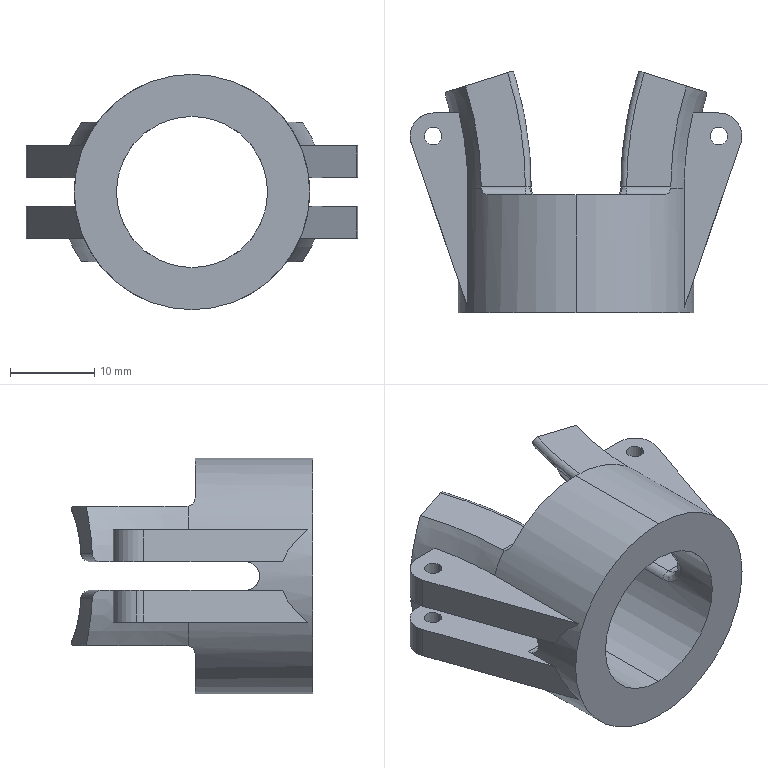Part | SolidWorks | features ICE 9, Fillet 4, MirrorPattern 4, Extrusion 1, Revolution 1 | 1 solid | 108 faces | box 39.5 x 28.723 x 28 mm | volume 7867 mm3 | cylinder 36 | plane 27 | spline 26 | torus 19 | commonest cylinder face diameters 2 x12 2.1 x8 5.5 x6 1.4 x4 3.4 x2 18 x2